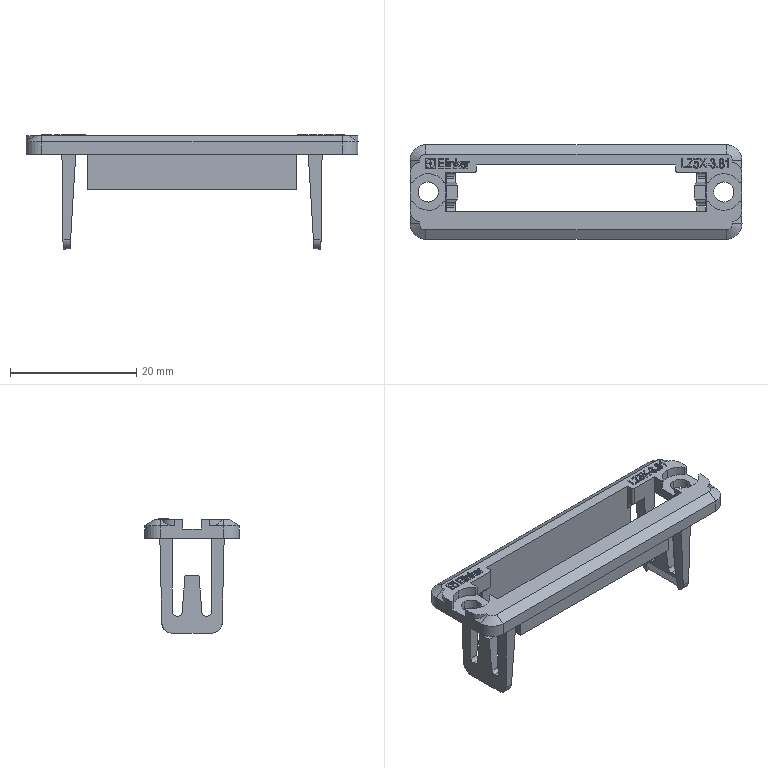Part | NX | features BREP 1 | 1 solid | 361 faces | box 52.67 x 15 x 18.1 mm | volume 1861 mm3 | plane 212 | spline 102 | cylinder 43 | cone 4 | commonest cylinder face diameters 3.2 x8 5.8 x8 1.2 x7 0.269 x4 4.035 x4 5 x4